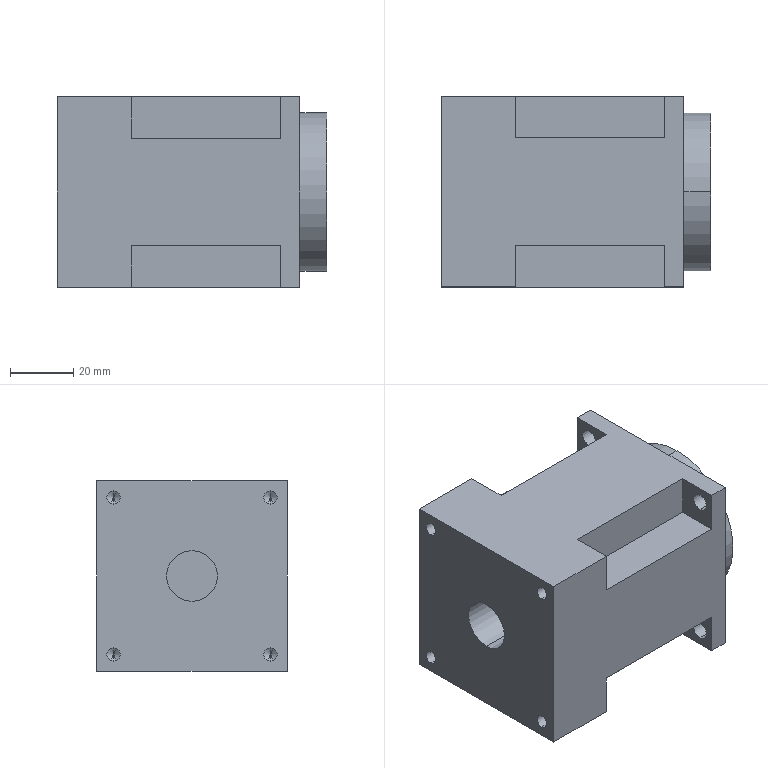Part | STEP file | 0245_Z_102_AB060-010-S1-P1_1 | 1 solid | 52 faces | box 85 x 60 x 60 mm | volume 252201 mm3 | plane 24 | cylinder 20 | cone 8 | commonest cylinder face diameters 4.2 x8 5.5 x8 16 x2 50 x2